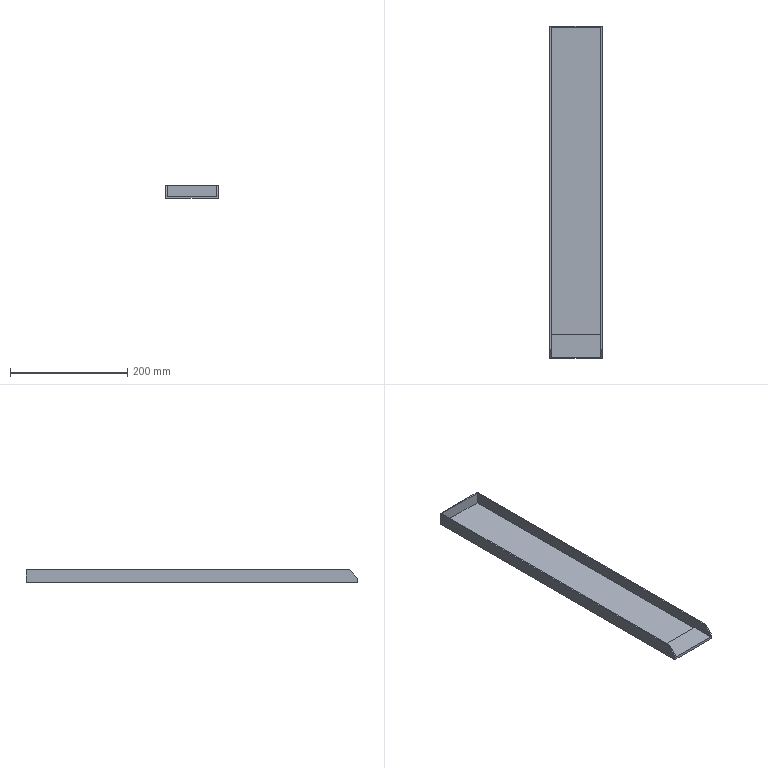Part | NX | features solid 2 | 1 solid | 14 faces | box 89 x 567 x 22 mm | volume 156036 mm3 | plane 14
STEP:
#1=CARTESIAN_POINT('',(-380.,-450.,-300.));
#2=VERTEX_POINT('',#1);
#3=CARTESIAN_POINT('',(-380.,102.,-300.));
#4=VERTEX_POINT('',#3);
#5=CARTESIAN_POINT('',(-380.,100.,-300.));
#6=DIRECTION('',(0.,-1.,0.));
#7=VECTOR('',#6,1000.);
#8=LINE('',#5,#7);
#9=EDGE_CURVE('',#2,#4,#8,.F.);
#10=ORIENTED_EDGE('',*,*,#9,.F.);
#11=CARTESIAN_POINT('',(-380.,-465.,-315.));
#12=VERTEX_POINT('',#11);
#13=CARTESIAN_POINT('',(-380.,-465.,-315.));
#14=DIRECTION('',(0.,-0.7071,-0.7071));
#15=VECTOR('',#14,1000.);
#16=LINE('',#13,#15);
#17=EDGE_CURVE('',#2,#12,#16,.T.);
#18=ORIENTED_EDGE('',*,*,#17,.T.);
#19=CARTESIAN_POINT('',(-380.,-465.,-322.));
#20=VERTEX_POINT('',#19);
#21=CARTESIAN_POINT('',(-380.,-465.,-320.));
#22=DIRECTION('',(0.,0.,-1.));
#23=VECTOR('',#22,1000.);
#24=LINE('',#21,#23);
#25=EDGE_CURVE('',#12,#20,#24,.T.);
#26=ORIENTED_EDGE('',*,*,#25,.T.);
#27=CARTESIAN_POINT('',(-380.,102.,-322.));
#28=VERTEX_POINT('',#27);
#29=CARTESIAN_POINT('',(-380.,-15.,-322.));
#30=DIRECTION('',(0.,-1.,0.));
#31=VECTOR('',#30,1000.);
#32=LINE('',#29,#31);
#33=EDGE_CURVE('',#20,#28,#32,.F.);
#34=ORIENTED_EDGE('',*,*,#33,.T.);
#35=CARTESIAN_POINT('',(-380.,102.,-320.));
#36=DIRECTION('',(0.,0.,-1.));
#37=VECTOR('',#36,1000.);
#38=LINE('',#35,#37);
#39=EDGE_CURVE('',#4,#28,#38,.T.);
#40=ORIENTED_EDGE('',*,*,#39,.F.);
#41=EDGE_LOOP('',(#10,#18,#26,#34,#40));
#42=FACE_BOUND('',#41,.T.);
#43=CARTESIAN_POINT('',(-380.,-15.,-320.));
#44=DIRECTION('',(-1.,0.,0.));
#45=DIRECTION('',(0.,0.,1.));
#46=AXIS2_PLACEMENT_3D('',#43,#44,#45);
#47=PLANE('',#46);
#48=ADVANCED_FACE('',(#42),#47,.F.);
#49=ORIENTED_EDGE('',*,*,#25,.F.);
#50=CARTESIAN_POINT('',(-382.,-465.,-315.));
#51=VERTEX_POINT('',#50);
#52=CARTESIAN_POINT('',(-910.,-465.,-315.));
#53=DIRECTION('',(-1.,0.,0.));
#54=VECTOR('',#53,1000.);
#55=LINE('',#52,#54);
#56=EDGE_CURVE('',#12,#51,#55,.T.);
#57=ORIENTED_EDGE('',*,*,#56,.T.);
#58=CARTESIAN_POINT('',(-382.,-465.,-318.));
#59=VERTEX_POINT('',#58);
#60=CARTESIAN_POINT('',(-382.,-465.,-320.));
#61=DIRECTION('',(0.,0.,-1.));
#62=VECTOR('',#61,1000.);
#63=LINE('',#60,#62);
#64=EDGE_CURVE('',#51,#59,#63,.T.);
#65=ORIENTED_EDGE('',*,*,#64,.T.);
#66=CARTESIAN_POINT('',(-467.,-465.,-318.));
#67=VERTEX_POINT('',#66);
#68=CARTESIAN_POINT('',(-483.,-465.,-318.));
#69=DIRECTION('',(-1.,0.,0.));
#70=VECTOR('',#69,1000.);
#71=LINE('',#68,#70);
#72=EDGE_CURVE('',#67,#59,#71,.F.);
#73=ORIENTED_EDGE('',*,*,#72,.F.);
#74=CARTESIAN_POINT('',(-467.,-465.,-315.));
#75=VERTEX_POINT('',#74);
#76=CARTESIAN_POINT('',(-467.,-465.,-320.));
#77=DIRECTION('',(0.,0.,-1.));
#78=VECTOR('',#77,1000.);
#79=LINE('',#76,#78);
#80=EDGE_CURVE('',#75,#67,#79,.T.);
#81=ORIENTED_EDGE('',*,*,#80,.F.);
#82=CARTESIAN_POINT('',(-469.,-465.,-315.));
#83=VERTEX_POINT('',#82);
#84=CARTESIAN_POINT('',(-910.,-465.,-315.));
#85=DIRECTION('',(-1.,0.,0.));
#86=VECTOR('',#85,1000.);
#87=LINE('',#84,#86);
#88=EDGE_CURVE('',#75,#83,#87,.T.);
#89=ORIENTED_EDGE('',*,*,#88,.T.);
#90=CARTESIAN_POINT('',(-469.,-465.,-322.));
#91=VERTEX_POINT('',#90);
#92=CARTESIAN_POINT('',(-469.,-465.,-320.));
#93=DIRECTION('',(0.,0.,-1.));
#94=VECTOR('',#93,1000.);
#95=LINE('',#92,#94);
#96=EDGE_CURVE('',#83,#91,#95,.T.);
#97=ORIENTED_EDGE('',*,*,#96,.T.);
#98=CARTESIAN_POINT('',(-910.,-465.,-322.));
#99=DIRECTION('',(1.,0.,0.));
#100=VECTOR('',#99,1000.);
#101=LINE('',#98,#100);
#102=EDGE_CURVE('',#91,#20,#101,.T.);
#103=ORIENTED_EDGE('',*,*,#102,.T.);
#104=EDGE_LOOP('',(#49,#57,#65,#73,#81,#89,#97,#103));
#105=FACE_BOUND('',#104,.T.);
#106=CARTESIAN_POINT('',(-910.,-465.,-320.));
#107=DIRECTION('',(0.,1.,0.));
#108=DIRECTION('',(0.,0.,1.));
#109=AXIS2_PLACEMENT_3D('',#106,#107,#108);
#110=PLANE('',#109);
#111=ADVANCED_FACE('',(#105),#110,.F.);
#112=ORIENTED_EDGE('',*,*,#96,.F.);
#113=CARTESIAN_POINT('',(-469.,-450.,-300.));
#114=VERTEX_POINT('',#113);
#115=CARTESIAN_POINT('',(-469.,-450.,-300.));
#116=DIRECTION('',(0.,0.7071,0.7071));
#117=VECTOR('',#116,1000.);
#118=LINE('',#115,#117);
#119=EDGE_CURVE('',#83,#114,#118,.T.);
#120=ORIENTED_EDGE('',*,*,#119,.T.);
#121=CARTESIAN_POINT('',(-469.,102.,-300.));
#122=VERTEX_POINT('',#121);
#123=CARTESIAN_POINT('',(-469.,580.,-300.));
#124=DIRECTION('',(0.,-1.,0.));
#125=VECTOR('',#124,1000.);
#126=LINE('',#123,#125);
#127=EDGE_CURVE('',#114,#122,#126,.F.);
#128=ORIENTED_EDGE('',*,*,#127,.T.);
#129=CARTESIAN_POINT('',(-469.,102.,-322.));
#130=VERTEX_POINT('',#129);
#131=CARTESIAN_POINT('',(-469.,102.,-320.));
#132=DIRECTION('',(0.,0.,-1.));
#133=VECTOR('',#132,1000.);
#134=LINE('',#131,#133);
#135=EDGE_CURVE('',#122,#130,#134,.T.);
#136=ORIENTED_EDGE('',*,*,#135,.T.);
#137=CARTESIAN_POINT('',(-469.,580.,-322.));
#138=DIRECTION('',(0.,1.,0.));
#139=VECTOR('',#138,1000.);
#140=LINE('',#137,#139);
#141=EDGE_CURVE('',#130,#91,#140,.F.);
#142=ORIENTED_EDGE('',*,*,#141,.T.);
#143=EDGE_LOOP('',(#112,#120,#128,#136,#142));
#144=FACE_BOUND('',#143,.T.);
#145=CARTESIAN_POINT('',(-469.,580.,-320.));
#146=DIRECTION('',(1.,0.,0.));
#147=DIRECTION('',(0.,0.,-1.));
#148=AXIS2_PLACEMENT_3D('',#145,#146,#147);
#149=PLANE('',#148);
#150=ADVANCED_FACE('',(#144),#149,.F.);
#151=CARTESIAN_POINT('',(-467.,-425.,-320.));
#152=VERTEX_POINT('',#151);
#153=CARTESIAN_POINT('',(-382.,-425.,-320.));
#154=VERTEX_POINT('',#153);
#155=CARTESIAN_POINT('',(-483.,-425.,-320.));
#156=DIRECTION('',(1.,0.,0.));
#157=VECTOR('',#156,1000.);
#158=LINE('',#155,#157);
#159=EDGE_CURVE('',#152,#154,#158,.T.);
#160=ORIENTED_EDGE('',*,*,#159,.T.);
#161=CARTESIAN_POINT('',(-382.,100.,-320.));
#162=VERTEX_POINT('',#161);
#163=CARTESIAN_POINT('',(-382.,-70.,-320.));
#164=DIRECTION('',(0.,1.,0.));
#165=VECTOR('',#164,1000.);
#166=LINE('',#163,#165);
#167=EDGE_CURVE('',#162,#154,#166,.F.);
#168=ORIENTED_EDGE('',*,*,#167,.F.);
#169=CARTESIAN_POINT('',(-467.,100.,-320.));
#170=VERTEX_POINT('',#169);
#171=CARTESIAN_POINT('',(-380.,100.,-320.));
#172=DIRECTION('',(-1.,0.,0.));
#173=VECTOR('',#172,1000.);
#174=LINE('',#171,#173);
#175=EDGE_CURVE('',#162,#170,#174,.T.);
#176=ORIENTED_EDGE('',*,*,#175,.T.);
#177=CARTESIAN_POINT('',(-467.,-70.,-320.));
#178=DIRECTION('',(0.,-1.,0.));
#179=VECTOR('',#178,1000.);
#180=LINE('',#177,#179);
#181=EDGE_CURVE('',#152,#170,#180,.F.);
#182=ORIENTED_EDGE('',*,*,#181,.F.);
#183=EDGE_LOOP('',(#160,#168,#176,#182));
#184=FACE_BOUND('',#183,.T.);
#185=CARTESIAN_POINT('',(-350.,-70.,-320.));
#186=DIRECTION('',(0.,0.,-1.));
#187=DIRECTION('',(-1.,0.,0.));
#188=AXIS2_PLACEMENT_3D('',#185,#186,#187);
#189=PLANE('',#188);
#190=ADVANCED_FACE('',(#184),#189,.F.);
#191=ORIENTED_EDGE('',*,*,#102,.F.);
#192=ORIENTED_EDGE('',*,*,#141,.F.);
#193=CARTESIAN_POINT('',(-380.,102.,-322.));
#194=DIRECTION('',(-1.,0.,0.));
#195=VECTOR('',#194,1000.);
#196=LINE('',#193,#195);
#197=EDGE_CURVE('',#28,#130,#196,.T.);
#198=ORIENTED_EDGE('',*,*,#197,.F.);
#199=ORIENTED_EDGE('',*,*,#33,.F.);
#200=EDGE_LOOP('',(#191,#192,#198,#199));
#201=FACE_BOUND('',#200,.T.);
#202=CARTESIAN_POINT('',(-350.,-70.,-322.));
#203=DIRECTION('',(0.,0.,-1.));
#204=DIRECTION('',(-1.,0.,0.));
#205=AXIS2_PLACEMENT_3D('',#202,#203,#204);
#206=PLANE('',#205);
#207=ADVANCED_FACE('',(#201),#206,.T.);
#208=CARTESIAN_POINT('',(-382.,100.,-300.));
#209=VERTEX_POINT('',#208);
#210=CARTESIAN_POINT('',(-382.,100.,-320.));
#211=DIRECTION('',(0.,0.,-1.));
#212=VECTOR('',#211,1000.);
#213=LINE('',#210,#212);
#214=EDGE_CURVE('',#209,#162,#213,.T.);
#215=ORIENTED_EDGE('',*,*,#214,.F.);
#216=CARTESIAN_POINT('',(-467.,100.,-300.));
#217=VERTEX_POINT('',#216);
#218=CARTESIAN_POINT('',(-380.,100.,-300.));
#219=DIRECTION('',(1.,0.,0.));
#220=VECTOR('',#219,1000.);
#221=LINE('',#218,#220);
#222=EDGE_CURVE('',#209,#217,#221,.F.);
#223=ORIENTED_EDGE('',*,*,#222,.T.);
#224=CARTESIAN_POINT('',(-467.,100.,-320.));
#225=DIRECTION('',(0.,0.,-1.));
#226=VECTOR('',#225,1000.);
#227=LINE('',#224,#226);
#228=EDGE_CURVE('',#217,#170,#227,.T.);
#229=ORIENTED_EDGE('',*,*,#228,.T.);
#230=ORIENTED_EDGE('',*,*,#175,.F.);
#231=EDGE_LOOP('',(#215,#223,#229,#230));
#232=FACE_BOUND('',#231,.T.);
#233=CARTESIAN_POINT('',(-380.,100.,-320.));
#234=DIRECTION('',(0.,-1.,0.));
#235=DIRECTION('',(0.,0.,-1.));
#236=AXIS2_PLACEMENT_3D('',#233,#234,#235);
#237=PLANE('',#236);
#238=ADVANCED_FACE('',(#232),#237,.T.);
#239=CARTESIAN_POINT('',(-382.,-450.,-300.));
#240=VERTEX_POINT('',#239);
#241=CARTESIAN_POINT('',(-382.,-15.,-300.));
#242=DIRECTION('',(0.,1.,0.));
#243=VECTOR('',#242,1000.);
#244=LINE('',#241,#243);
#245=EDGE_CURVE('',#240,#209,#244,.T.);
#246=ORIENTED_EDGE('',*,*,#245,.F.);
#247=CARTESIAN_POINT('',(-380.,-450.,-300.));
#248=DIRECTION('',(-1.,0.,0.));
#249=VECTOR('',#248,1000.);
#250=LINE('',#247,#249);
#251=EDGE_CURVE('',#240,#2,#250,.F.);
#252=ORIENTED_EDGE('',*,*,#251,.T.);
#253=ORIENTED_EDGE('',*,*,#9,.T.);
#254=CARTESIAN_POINT('',(-380.,102.,-300.));
#255=DIRECTION('',(1.,0.,0.));
#256=VECTOR('',#255,1000.);
#257=LINE('',#254,#256);
#258=EDGE_CURVE('',#4,#122,#257,.F.);
#259=ORIENTED_EDGE('',*,*,#258,.T.);
#260=ORIENTED_EDGE('',*,*,#127,.F.);
#261=CARTESIAN_POINT('',(-467.,-450.,-300.));
#262=VERTEX_POINT('',#261);
#263=CARTESIAN_POINT('',(-380.,-450.,-300.));
#264=DIRECTION('',(-1.,0.,0.));
#265=VECTOR('',#264,1000.);
#266=LINE('',#263,#265);
#267=EDGE_CURVE('',#114,#262,#266,.F.);
#268=ORIENTED_EDGE('',*,*,#267,.T.);
#269=CARTESIAN_POINT('',(-467.,-15.,-300.));
#270=DIRECTION('',(0.,1.,0.));
#271=VECTOR('',#270,1000.);
#272=LINE('',#269,#271);
#273=EDGE_CURVE('',#217,#262,#272,.F.);
#274=ORIENTED_EDGE('',*,*,#273,.F.);
#275=ORIENTED_EDGE('',*,*,#222,.F.);
#276=EDGE_LOOP('',(#246,#252,#253,#259,#260,#268,#274,#275));
#277=FACE_BOUND('',#276,.T.);
#278=CARTESIAN_POINT('',(-380.,-15.,-300.));
#279=DIRECTION('',(0.,0.,1.));
#280=DIRECTION('',(1.,0.,0.));
#281=AXIS2_PLACEMENT_3D('',#278,#279,#280);
#282=PLANE('',#281);
#283=ADVANCED_FACE('',(#277),#282,.T.);
#284=ORIENTED_EDGE('',*,*,#197,.T.);
#285=ORIENTED_EDGE('',*,*,#135,.F.);
#286=ORIENTED_EDGE('',*,*,#258,.F.);
#287=ORIENTED_EDGE('',*,*,#39,.T.);
#288=EDGE_LOOP('',(#284,#285,#286,#287));
#289=FACE_BOUND('',#288,.T.);
#290=CARTESIAN_POINT('',(-380.,102.,-320.));
#291=DIRECTION('',(0.,-1.,0.));
#292=DIRECTION('',(0.,0.,-1.));
#293=AXIS2_PLACEMENT_3D('',#290,#291,#292);
#294=PLANE('',#293);
#295=ADVANCED_FACE('',(#289),#294,.F.);
#296=ORIENTED_EDGE('',*,*,#273,.T.);
#297=CARTESIAN_POINT('',(-467.,55.,205.));
#298=DIRECTION('',(0.,-0.7071,-0.7071));
#299=VECTOR('',#298,1000.);
#300=LINE('',#297,#299);
#301=EDGE_CURVE('',#262,#75,#300,.T.);
#302=ORIENTED_EDGE('',*,*,#301,.T.);
#303=ORIENTED_EDGE('',*,*,#80,.T.);
#304=CARTESIAN_POINT('',(-467.,-425.,-318.));
#305=VERTEX_POINT('',#304);
#306=CARTESIAN_POINT('',(-467.,-425.,-318.));
#307=DIRECTION('',(0.,-1.,0.));
#308=VECTOR('',#307,1000.);
#309=LINE('',#306,#308);
#310=EDGE_CURVE('',#305,#67,#309,.T.);
#311=ORIENTED_EDGE('',*,*,#310,.F.);
#312=CARTESIAN_POINT('',(-467.,-425.,-320.));
#313=DIRECTION('',(0.,0.,1.));
#314=VECTOR('',#313,1000.);
#315=LINE('',#312,#314);
#316=EDGE_CURVE('',#152,#305,#315,.T.);
#317=ORIENTED_EDGE('',*,*,#316,.F.);
#318=ORIENTED_EDGE('',*,*,#181,.T.);
#319=ORIENTED_EDGE('',*,*,#228,.F.);
#320=EDGE_LOOP('',(#296,#302,#303,#311,#317,#318,#319));
#321=FACE_BOUND('',#320,.T.);
#322=CARTESIAN_POINT('',(-467.,580.,-320.));
#323=DIRECTION('',(1.,0.,0.));
#324=DIRECTION('',(0.,0.,-1.));
#325=AXIS2_PLACEMENT_3D('',#322,#323,#324);
#326=PLANE('',#325);
#327=ADVANCED_FACE('',(#321),#326,.T.);
#328=ORIENTED_EDGE('',*,*,#64,.F.);
#329=CARTESIAN_POINT('',(-382.,-242.5,-92.5));
#330=DIRECTION('',(0.,0.7071,0.7071));
#331=VECTOR('',#330,1000.);
#332=LINE('',#329,#331);
#333=EDGE_CURVE('',#51,#240,#332,.T.);
#334=ORIENTED_EDGE('',*,*,#333,.T.);
#335=ORIENTED_EDGE('',*,*,#245,.T.);
#336=ORIENTED_EDGE('',*,*,#214,.T.);
#337=ORIENTED_EDGE('',*,*,#167,.T.);
#338=CARTESIAN_POINT('',(-382.,-425.,-318.));
#339=VERTEX_POINT('',#338);
#340=CARTESIAN_POINT('',(-382.,-425.,-320.));
#341=DIRECTION('',(0.,0.,1.));
#342=VECTOR('',#341,1000.);
#343=LINE('',#340,#342);
#344=EDGE_CURVE('',#154,#339,#343,.T.);
#345=ORIENTED_EDGE('',*,*,#344,.T.);
#346=CARTESIAN_POINT('',(-382.,-425.,-318.));
#347=DIRECTION('',(0.,1.,0.));
#348=VECTOR('',#347,1000.);
#349=LINE('',#346,#348);
#350=EDGE_CURVE('',#339,#59,#349,.F.);
#351=ORIENTED_EDGE('',*,*,#350,.T.);
#352=EDGE_LOOP('',(#328,#334,#335,#336,#337,#345,#351));
#353=FACE_BOUND('',#352,.T.);
#354=CARTESIAN_POINT('',(-382.,-15.,-320.));
#355=DIRECTION('',(-1.,0.,0.));
#356=DIRECTION('',(0.,0.,1.));
#357=AXIS2_PLACEMENT_3D('',#354,#355,#356);
#358=PLANE('',#357);
#359=ADVANCED_FACE('',(#353),#358,.T.);
#360=ORIENTED_EDGE('',*,*,#344,.F.);
#361=ORIENTED_EDGE('',*,*,#159,.F.);
#362=ORIENTED_EDGE('',*,*,#316,.T.);
#363=CARTESIAN_POINT('',(-483.,-425.,-318.));
#364=DIRECTION('',(-1.,0.,0.));
#365=VECTOR('',#364,1000.);
#366=LINE('',#363,#365);
#367=EDGE_CURVE('',#305,#339,#366,.F.);
#368=ORIENTED_EDGE('',*,*,#367,.T.);
#369=EDGE_LOOP('',(#360,#361,#362,#368));
#370=FACE_BOUND('',#369,.T.);
#371=CARTESIAN_POINT('',(-483.,-425.,-320.));
#372=DIRECTION('',(0.,1.,0.));
#373=DIRECTION('',(1.,0.,0.));
#374=AXIS2_PLACEMENT_3D('',#371,#372,#373);
#375=PLANE('',#374);
#376=ADVANCED_FACE('',(#370),#375,.T.);
#377=ORIENTED_EDGE('',*,*,#72,.T.);
#378=ORIENTED_EDGE('',*,*,#350,.F.);
#379=ORIENTED_EDGE('',*,*,#367,.F.);
#380=ORIENTED_EDGE('',*,*,#310,.T.);
#381=EDGE_LOOP('',(#377,#378,#379,#380));
#382=FACE_BOUND('',#381,.T.);
#383=CARTESIAN_POINT('',(-483.,-425.,-318.));
#384=DIRECTION('',(0.,0.,-1.));
#385=DIRECTION('',(-1.,0.,0.));
#386=AXIS2_PLACEMENT_3D('',#383,#384,#385);
#387=PLANE('',#386);
#388=ADVANCED_FACE('',(#382),#387,.F.);
#389=ORIENTED_EDGE('',*,*,#119,.F.);
#390=ORIENTED_EDGE('',*,*,#88,.F.);
#391=ORIENTED_EDGE('',*,*,#301,.F.);
#392=ORIENTED_EDGE('',*,*,#267,.F.);
#393=EDGE_LOOP('',(#389,#390,#391,#392));
#394=FACE_BOUND('',#393,.T.);
#395=CARTESIAN_POINT('',(-380.,-450.,-300.));
#396=DIRECTION('',(0.,-0.7071,0.7071));
#397=DIRECTION('',(0.,-0.7071,-0.7071));
#398=AXIS2_PLACEMENT_3D('',#395,#396,#397);
#399=PLANE('',#398);
#400=ADVANCED_FACE('',(#394),#399,.T.);
#401=ORIENTED_EDGE('',*,*,#17,.F.);
#402=ORIENTED_EDGE('',*,*,#251,.F.);
#403=ORIENTED_EDGE('',*,*,#333,.F.);
#404=ORIENTED_EDGE('',*,*,#56,.F.);
#405=EDGE_LOOP('',(#401,#402,#403,#404));
#406=FACE_BOUND('',#405,.T.);
#407=CARTESIAN_POINT('',(-910.,-465.,-315.));
#408=DIRECTION('',(0.,-0.7071,0.7071));
#409=DIRECTION('',(0.,-0.7071,-0.7071));
#410=AXIS2_PLACEMENT_3D('',#407,#408,#409);
#411=PLANE('',#410);
#412=ADVANCED_FACE('',(#406),#411,.T.);
#413=CLOSED_SHELL('',(#48,#111,#150,#190,#207,#238,#283,#295,#327,#359,#376,#388,#400,#412));
#414=MANIFOLD_SOLID_BREP('',#413);
#415=(LENGTH_UNIT()NAMED_UNIT(*)SI_UNIT(.MILLI.,.METRE.));
#416=UNCERTAINTY_MEASURE_WITH_UNIT(LENGTH_MEASURE(0.00001),#415,'','');
#417=(NAMED_UNIT(*)PLANE_ANGLE_UNIT()SI_UNIT($,.RADIAN.));
#418=(NAMED_UNIT(*)SI_UNIT($,.STERADIAN.)SOLID_ANGLE_UNIT());
#419=(GEOMETRIC_REPRESENTATION_CONTEXT(3)GLOBAL_UNCERTAINTY_ASSIGNED_CONTEXT((#416))GLOBAL_UNIT_ASSIGNED_CONTEXT((#415,#417,#418))REPRESENTATION_CONTEXT('',''));
#420=ADVANCED_BREP_SHAPE_REPRESENTATION('',(#414),#419);